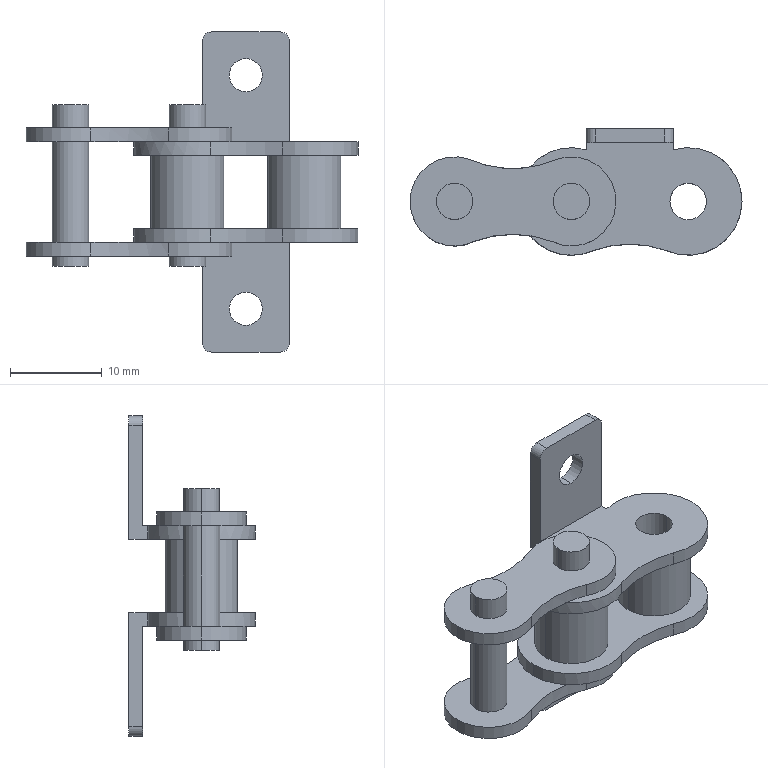Part | STEP file | CHEL40Achain | 1 solid | 64 faces | box 36.1 x 13.75 x 34.8 mm | volume 2522 mm3 | cylinder 42 | plane 22 | commonest cylinder face diameters 3.97 x12 9.7 x6 11.7 x6 23.4 x6 2 x4 3.6 x4